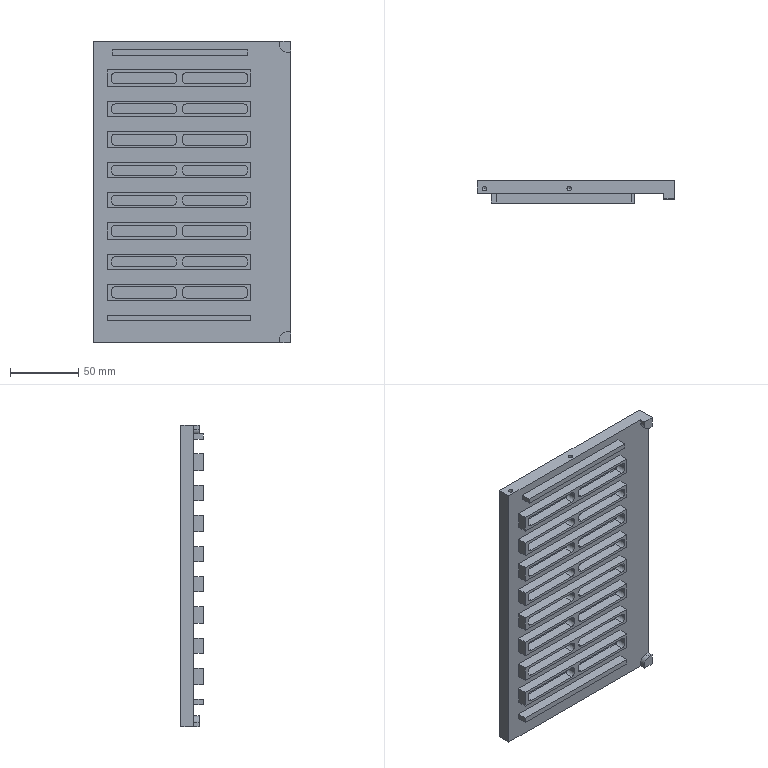NC program | NX | posted with a generic post | part box 144.5 x 16.5 x 221 mm
Lines 4750 to 5825 of 11164:
(CAVITY_MILL_COPY , TOOL : D5-15-D6-50-3T-ROUGH)
N9486 T03 M6
N9488 G54
N9490 G17 G0 G90 X82. Y-0.207 B0. C0. S4500 M3
N9492 G43 Z20. H3
N9494 Z0.533 B-180. C-180.
N9496 G94 G1 Y4.25 Z0.378 F1200.
N9498 Y4.387 Z0.373
N9500 X82.163 Y4.55 Z0.365
N9502 X82.3 Z0.36
N9504 X84.514 Z0.283
N9506 X84.583 Y4.546 Z0.28
N9508 X84.644 Y4.513 Z0.278
N9510 X84.763 Y4.394 Z0.272
N9512 X84.8 Y4.327 Z0.269
N9514 Y-10.463 Z-0.247
N9516 Y-16.75 Z-0.467
N9518 Y-37.75
N9520 X84.79 Y-37.826
N9522 G2 X84.465 Y-38.05 R0.302
N9524 G1 X82.335
N9526 G2 X82.105 Y-37.978 R0.409
N9528 X82. Y-37.75 R0.3
N9530 G1 Y4.25
N9532 G2 X82.3 Y4.55 R0.3
N9534 G1 X84.514
N9536 X84.589 Y4.568
N9538 X84.644 Y4.513
N9540 X84.763 Y4.394
N9542 X84.82 Y4.332
N9544 X84.8 Y4.25
N9546 Y-16.75
N9548 Z0.533
N9550 G0 Z20.
N9552 X82. Y-0.206
N9554 Z0.067
N9556 G1 Y4.387 Z-0.094
N9558 X82.163 Y4.55 Z-0.102
N9560 X84.577 Z-0.186
N9562 X84.644 Y4.513 Z-0.189
N9564 X84.763 Y4.394 Z-0.195
N9566 X84.8 Y4.327 Z-0.197
N9568 Y-16.75 Z-0.933
N9570 Y-37.75
N9572 X84.79 Y-37.825
N9574 G2 X84.5 Y-38.05 R0.3
N9576 G1 X82.335
N9578 G2 X82.105 Y-37.978 R0.409
N9580 X82. Y-37.75 R0.3
N9582 G1 Y4.25
N9584 G2 X82.3 Y4.55 R0.3
N9586 G1 X84.5
N9588 X84.582 Y4.57
N9590 X84.644 Y4.513
N9592 X84.763 Y4.394
N9594 X84.82 Y4.332
N9596 X84.8 Y4.25
N9598 Y-16.75
N9600 Z0.067
N9602 G0 Z20.
N9604 X82. Y-0.206
N9606 Z-0.4
N9608 G1 Y4.25 Z-0.556
N9610 Y4.387 Z-0.56
N9612 X82.163 Y4.55 Z-0.568
N9614 X82.3 Z-0.573
N9616 X84.577 Z-0.653
N9618 X84.644 Y4.513 Z-0.655
N9620 X84.763 Y4.394 Z-0.661
N9622 X84.8 Y4.327 Z-0.664
N9624 Y-16.75 Z-1.4
N9626 Y-37.75
N9628 X84.79 Y-37.825
N9630 G2 X84.5 Y-38.05 R0.3
N9632 G1 X82.335
N9634 G2 X82.105 Y-37.978 R0.409
N9636 X82. Y-37.75 R0.3
N9638 G1 Y4.25
N9640 G2 X82.3 Y4.55 R0.3
N9642 G1 X84.5
N9644 X84.582 Y4.57
N9646 X84.644 Y4.513
N9648 X84.763 Y4.394
N9650 X84.82 Y4.332
N9652 X84.8 Y4.25
N9654 Y-16.75
N9656 Z-0.4
N9658 G0 Z20.
N9660 X82. Y-0.206
N9662 Z-0.867
N9664 G1 Y4.25 Z-1.022
N9666 Y4.387 Z-1.027
N9668 X82.163 Y4.55 Z-1.035
N9670 X82.3 Z-1.04
N9672 X84.577 Z-1.119
N9674 X84.644 Y4.513 Z-1.122
N9676 X84.763 Y4.394 Z-1.128
N9678 X84.8 Y4.327 Z-1.131
N9680 Y-16.75 Z-1.867
N9682 Y-37.75
N9684 X84.79 Y-37.825
N9686 G2 X84.5 Y-38.05 R0.3
N9688 G1 X82.335
N9690 G2 X82.105 Y-37.978 R0.409
N9692 X82. Y-37.75 R0.3
N9694 G1 Y4.25
N9696 G2 X82.3 Y4.55 R0.3
N9698 G1 X84.5
N9700 X84.582 Y4.57
N9702 X84.644 Y4.513
N9704 X84.763 Y4.394
N9706 X84.82 Y4.332
N9708 X84.8 Y4.25
N9710 Y-16.75
N9712 Z-0.867
N9714 G0 Z20.
N9716 X82. Y-0.206
N9718 Z-1.333
N9720 G1 Y4.387 Z-1.494
N9722 X82.163 Y4.55 Z-1.502
N9724 X84.577 Z-1.586
N9726 X84.644 Y4.513 Z-1.589
N9728 X84.763 Y4.394 Z-1.595
N9730 X84.8 Y4.327 Z-1.597
N9732 Y-16.75 Z-2.333
N9734 Y-37.75
N9736 X84.79 Y-37.825
N9738 G2 X84.5 Y-38.05 R0.3
N9740 G1 X82.335
N9742 G2 X82.105 Y-37.978 R0.409
N9744 X82. Y-37.75 R0.3
N9746 G1 Y4.25
N9748 G2 X82.3 Y4.55 R0.3
N9750 G1 X84.5
N9752 X84.582 Y4.57
N9754 X84.644 Y4.513
N9756 X84.763 Y4.394
N9758 X84.82 Y4.332
N9760 X84.8 Y4.25
N9762 Y-16.75
N9764 Z-1.333
N9766 G0 Z20.
N9768 X82. Y-0.206
N9770 Z-1.8
N9772 G1 Y4.387 Z-1.96
N9774 X82.163 Y4.55 Z-1.968
N9776 X84.577 Z-2.053
N9778 X84.644 Y4.513 Z-2.055
N9780 X84.763 Y4.394 Z-2.061
N9782 X84.8 Y4.327 Z-2.064
N9784 Y-16.75 Z-2.8
N9786 Y-37.75
N9788 X84.79 Y-37.825
N9790 G2 X84.5 Y-38.05 R0.3
N9792 G1 X82.335
N9794 G2 X82.105 Y-37.978 R0.409
N9796 X82. Y-37.75 R0.3
N9798 G1 Y4.25
N9800 G2 X82.3 Y4.55 R0.3
N9802 G1 X84.5
N9804 X84.582 Y4.57
N9806 X84.644 Y4.513
N9808 X84.763 Y4.394
N9810 X84.82 Y4.332
N9812 X84.8 Y4.25
N9814 Y-16.75
N9816 Z-1.8
N9818 G0 Z20.
N9820 X82. Y-0.206
N9822 Z-2.3
N9824 G1 Y4.25 Z-2.456
N9826 Y4.387 Z-2.46
N9828 X82.163 Y4.55 Z-2.468
N9830 X82.3 Z-2.473
N9832 X84.577 Z-2.553
N9834 X84.644 Y4.513 Z-2.555
N9836 X84.763 Y4.394 Z-2.561
N9838 X84.8 Y4.327 Z-2.564
N9840 Y-16.75 Z-3.3
N9842 Y-37.75
N9844 X84.79 Y-37.825
N9846 G2 X84.5 Y-38.05 R0.3
N9848 G1 X82.335
N9850 G2 X82.105 Y-37.978 R0.409
N9852 G1 X82.06 Y-37.93
N9854 X81.987 Y-37.855
N9856 X82. Y-37.75
N9858 Y4.25
N9860 G2 X82.3 Y4.55 R0.3
N9862 G1 X84.5
N9864 X84.582 Y4.57
N9866 X84.644 Y4.513
N9868 X84.763 Y4.394
N9870 X84.82 Y4.332
N9872 X84.8 Y4.25
N9874 Y-16.75
N9876 Z-2.3
N9878 G0 Z20.
N9880 X82. Y-0.206
N9882 Z-2.8
N9884 G1 Y4.387 Z-2.96
N9886 X82.163 Y4.55 Z-2.968
N9888 X84.577 Z-3.053
N9890 X84.644 Y4.513 Z-3.055
N9892 X84.763 Y4.394 Z-3.061
N9894 X84.8 Y4.327 Z-3.064
N9896 Y-16.75 Z-3.8
N9898 Y-37.75
N9900 X84.79 Y-37.825
N9902 G2 X84.5 Y-38.05 R0.3
N9904 G1 X82.335
N9906 G2 X82.105 Y-37.978 R0.409
N9908 X82. Y-37.75 R0.3
N9910 G1 Y4.25
N9912 G2 X82.3 Y4.55 R0.3
N9914 G1 X84.5
N9916 X84.582 Y4.57
N9918 X84.644 Y4.513
N9920 X84.763 Y4.394
N9922 X84.82 Y4.332
N9924 X84.8 Y4.25
N9926 Y-16.75
N9928 Z-2.8
N9930 G0 Z20.
N9932 X82. Y-0.206
N9934 Z-3.3
N9936 G1 Y4.387 Z-3.46
N9938 X82.163 Y4.55 Z-3.468
N9940 X84.577 Z-3.553
N9942 X84.644 Y4.513 Z-3.555
N9944 X84.763 Y4.394 Z-3.561
N9946 X84.8 Y4.327 Z-3.564
N9948 Y-16.75 Z-4.3
N9950 Y-37.75
N9952 X84.79 Y-37.825
N9954 G2 X84.5 Y-38.05 R0.3
N9956 G1 X82.335
N9958 G2 X82.105 Y-37.978 R0.409
N9960 X82. Y-37.75 R0.3
N9962 G1 Y4.25
N9964 G2 X82.3 Y4.55 R0.3
N9966 G1 X84.5
N9968 X84.582 Y4.57
N9970 X84.644 Y4.513
N9972 X84.763 Y4.394
N9974 X84.82 Y4.332
N9976 X84.8 Y4.25
N9978 Y-16.75
N9980 Z-3.3
N9982 G0 Z20.
N9984 X82. Y-0.206
N9986 Z-3.8
N9988 G1 Y4.387 Z-3.96
N9990 X82.163 Y4.55 Z-3.968
N9992 X84.577 Z-4.053
N9994 X84.644 Y4.513 Z-4.055
N9996 X84.763 Y4.394 Z-4.061
N9998 X84.8 Y4.327 Z-4.064
N10000 Y-16.75 Z-4.8
N10002 Y-37.75
N10004 X84.79 Y-37.825
N10006 G2 X84.5 Y-38.05 R0.3
N10008 G1 X82.335
N10010 G2 X82.105 Y-37.978 R0.409
N10012 X82. Y-37.75 R0.3
N10014 G1 Y4.25
N10016 G2 X82.3 Y4.55 R0.3
N10018 G1 X84.5
N10020 X84.582 Y4.57
N10022 X84.644 Y4.513
N10024 X84.763 Y4.394
N10026 X84.82 Y4.332
N10028 X84.8 Y4.25
N10030 Y-16.75
N10032 Z-3.8
N10034 G0 Z20.
N10036 X82. Y-0.206
N10038 Z-4.3
N10040 G1 Y4.387 Z-4.46
N10042 X82.163 Y4.55 Z-4.468
N10044 X84.577 Z-4.553
N10046 X84.644 Y4.513 Z-4.555
N10048 X84.763 Y4.394 Z-4.561
N10050 X84.8 Y4.327 Z-4.564
N10052 Y-16.75 Z-5.3
N10054 Y-37.75
N10056 X84.79 Y-37.825
N10058 G2 X84.5 Y-38.05 R0.3
N10060 G1 X82.335
N10062 G2 X82.105 Y-37.978 R0.409
N10064 X82. Y-37.75 R0.3
N10066 G1 Y4.25
N10068 G2 X82.3 Y4.55 R0.3
N10070 G1 X84.5
N10072 X84.582 Y4.57
N10074 X84.644 Y4.513
N10076 X84.763 Y4.394
N10078 X84.82 Y4.332
N10080 X84.8 Y4.25
N10082 Y-16.75
N10084 Z-4.3
N10086 G0 Z20.
N10088 X82. Y-0.206
N10090 Z-4.8
N10092 G1 Y4.387 Z-4.96
N10094 X82.163 Y4.55 Z-4.968
N10096 X84.577 Z-5.053
N10098 X84.644 Y4.513 Z-5.055
N10100 X84.763 Y4.394 Z-5.061
N10102 X84.8 Y4.327 Z-5.064
N10104 Y-16.75 Z-5.8
N10106 Y-37.75
N10108 X84.79 Y-37.825
N10110 G2 X84.5 Y-38.05 R0.3
N10112 G1 X82.334
N10114 G2 X82.105 Y-37.978 R0.409
N10116 X82. Y-37.75 R0.3
N10118 G1 Y4.25
N10120 G2 X82.3 Y4.55 R0.3
N10122 G1 X84.5
N10124 X84.582 Y4.57
N10126 X84.644 Y4.513
N10128 X84.763 Y4.394
N10130 X84.82 Y4.332
N10132 X84.8 Y4.25
N10134 Y-16.75
N10136 Z-4.8
N10138 G0 Z20.
N10140 X82. Y-0.206
N10142 Z-5.3
N10144 G1 Y4.387 Z-5.46
N10146 X82.163 Y4.55 Z-5.468
N10148 X84.577 Z-5.553
N10150 X84.644 Y4.513 Z-5.555
N10152 X84.763 Y4.394 Z-5.561
N10154 X84.8 Y4.327 Z-5.564
N10156 Y-16.75 Z-6.3
N10158 Y-37.75
N10160 X84.79 Y-37.825
N10162 G2 X84.5 Y-38.05 R0.3
N10164 G1 X82.334
N10166 G2 X82.105 Y-37.978 R0.409
N10168 X82. Y-37.75 R0.3
N10170 G1 Y4.25
N10172 G2 X82.3 Y4.55 R0.3
N10174 G1 X84.5
N10176 X84.582 Y4.57
N10178 X84.644 Y4.513
N10180 X84.763 Y4.394
N10182 X84.82 Y4.332
N10184 X84.8 Y4.25
N10186 Y-16.75
N10188 Z-5.3
N10190 G0 Z20.
N10192 X82. Y-0.206
N10194 Z-5.8
N10196 G1 Y4.387 Z-5.96
N10198 X82.163 Y4.55 Z-5.968
N10200 X84.577 Z-6.053
N10202 X84.644 Y4.513 Z-6.055
N10204 X84.763 Y4.394 Z-6.061
N10206 X84.8 Y4.327 Z-6.064
N10208 Y-16.75 Z-6.8
N10210 Y-37.75
N10212 X84.79 Y-37.825
N10214 G2 X84.5 Y-38.05 R0.3
N10216 G1 X82.334
N10218 G2 X82.105 Y-37.978 R0.409
N10220 X82. Y-37.75 R0.3
N10222 G1 Y4.25
N10224 G2 X82.3 Y4.55 R0.3
N10226 G1 X84.5
N10228 X84.582 Y4.57
N10230 X84.644 Y4.513
N10232 X84.763 Y4.394
N10234 X84.82 Y4.332
N10236 X84.8 Y4.25
N10238 Y-16.75
N10240 Z-5.8
N10242 G0 Z20.
N10244 X61.8 Y-32.367
N10246 Z0.533
N10248 G1 Y-37.75 Z0.345
N10250 Y-37.887 Z0.341
N10252 X61.638 Y-38.05 Z0.333
N10254 X61.501 Z0.328
N10256 X61.261 Z0.319
N10258 X60.259 Y-38.047 Z0.284
N10260 X60.12 Y-38.023 Z0.279
N10262 X60.027 Y-37.93 Z0.275
N10264 X60. Y-37.771 Z0.269
N10266 Y-16.697 Z-0.467
N10268 Y4.25
N10270 X60.036 Y4.392
N10272 G2 X60.3 Y4.55 R0.3
N10274 G1 X61.5
N10276 G2 X61.8 Y4.25 R0.3
N10278 G1 Y-37.75
N10280 G2 X61.501 Y-38.05 R0.3
N10282 G1 X61.261
N10284 X60.259 Y-38.047
N10286 G2 X60. Y-37.75 R0.316
N10288 G1 Y-16.697
N10290 Z0.533
N10292 G0 Z20.
N10294 X61.8 Y-32.367
N10296 Z0.067
N10298 G1 Y-37.75 Z-0.121
N10300 Y-37.887 Z-0.126
N10302 X61.638 Y-38.05 Z-0.134
N10304 X61.501 Z-0.139
N10306 X61.301 Z-0.146
N10308 X60.259 Y-38.047 Z-0.182
N10310 X60.12 Y-38.023 Z-0.187
N10312 X60.027 Y-37.93 Z-0.192
N10314 X60. Y-37.771 Z-0.197
N10316 Y-16.697 Z-0.933
N10318 Y4.25
N10320 X60.036 Y4.392
N10322 G2 X60.3 Y4.55 R0.3
N10324 G1 X61.5
N10326 G2 X61.8 Y4.25 R0.3
N10328 G1 Y-37.75
N10330 G2 X61.501 Y-38.05 R0.3
N10332 G1 X61.301
N10334 X60.259 Y-38.047
N10336 G2 X60. Y-37.75 R0.316
N10338 G1 Y-16.697
N10340 Z0.067
N10342 G0 Z20.
N10344 X61.8 Y-32.367
N10346 Z-0.4
N10348 G1 Y-37.75 Z-0.588
N10350 Y-37.887 Z-0.593
N10352 X61.638 Y-38.05 Z-0.601
N10354 X61.5 Z-0.606
N10356 X61.341 Z-0.611
N10358 X60.259 Y-38.047 Z-0.649
N10360 X60.12 Y-38.023 Z-0.654
N10362 X60.027 Y-37.93 Z-0.658
N10364 X60. Y-37.771 Z-0.664
N10366 Y-16.697 Z-1.4
N10368 Y4.25
N10370 X60.036 Y4.392
N10372 G2 X60.3 Y4.55 R0.3
N10374 G1 X61.5
N10376 G2 X61.8 Y4.25 R0.3
N10378 G1 Y-37.75
N10380 G2 X61.5 Y-38.05 R0.3
N10382 G1 X61.341
N10384 X60.259 Y-38.047
N10386 G2 X60. Y-37.75 R0.316
N10388 G1 Y-16.697
N10390 Z-0.4
N10392 G0 Z20.
N10394 X61.8 Y-32.367
N10396 Z-0.867
N10398 G1 Y-37.75 Z-1.055
N10400 Y-37.887 Z-1.059
N10402 X61.638 Y-38.05 Z-1.067
N10404 X61.5 Z-1.072
N10406 X61.381 Z-1.076
N10408 X60.259 Y-38.047 Z-1.116
N10410 X60.12 Y-38.023 Z-1.121
N10412 X60.027 Y-37.93 Z-1.125
N10414 X60. Y-37.771 Z-1.131
N10416 Y-16.697 Z-1.867
N10418 Y4.25
N10420 X60.036 Y4.392
N10422 G2 X60.3 Y4.55 R0.3
N10424 G1 X61.5
N10426 G2 X61.8 Y4.25 R0.3
N10428 G1 Y-37.75
N10430 G2 X61.5 Y-38.05 R0.3
N10432 G1 X61.381
N10434 X60.259 Y-38.047
N10436 G2 X60. Y-37.75 R0.316
N10438 G1 Y-16.697
N10440 Z-0.867
N10442 G0 Z20.
N10444 X61.8 Y-32.367
N10446 Z-1.333
N10448 G1 Y-37.75 Z-1.521
N10450 Y-37.887 Z-1.526
N10452 X61.638 Y-38.05 Z-1.534
N10454 X61.5 Z-1.539
N10456 X61.421 Z-1.542
N10458 X60.259 Y-38.047 Z-1.582
N10460 X60.12 Y-38.023 Z-1.587
N10462 X60.027 Y-37.93 Z-1.592
N10464 X60. Y-37.771 Z-1.597
N10466 Y-16.697 Z-2.333
N10468 Y4.25
N10470 X60.036 Y4.392
N10472 G2 X60.3 Y4.55 R0.3
N10474 G1 X61.5
N10476 G2 X61.8 Y4.25 R0.3
N10478 G1 Y-37.75
N10480 G2 X61.5 Y-38.05 R0.3
N10482 G1 X61.421
N10484 X60.259 Y-38.047
N10486 G2 X60. Y-37.75 R0.316
N10488 G1 Y-16.697
N10490 Z-1.333
N10492 G0 Z20.
N10494 X61.8 Y-32.367
N10496 Z-1.8
N10498 G1 Y-37.75 Z-1.988
N10500 Y-37.887 Z-1.993
N10502 X61.638 Y-38.05 Z-2.001
N10504 X61.46 Z-2.007
N10506 X60.259 Y-38.047 Z-2.049
N10508 X60.12 Y-38.023 Z-2.054
N10510 X60.027 Y-37.93 Z-2.058
N10512 X60. Y-37.771 Z-2.064
N10514 Y-16.697 Z-2.8
N10516 Y4.25
N10518 X60.036 Y4.392
N10520 G2 X60.3 Y4.55 R0.3
N10522 G1 X61.5
N10524 G2 X61.8 Y4.25 R0.3
N10526 G1 Y-37.75
N10528 G2 X61.46 Y-38.05 R0.303
N10530 G1 X60.259 Y-38.047
N10532 G2 X60. Y-37.75 R0.316
N10534 G1 Y-16.697
N10536 Z-1.8
N10538 G0 Z20.
N10540 X61.8 Y-32.366
N10542 Z-2.3
N10544 G1 Y-37.75 Z-2.488
N10546 Y-37.887 Z-2.493
N10548 X61.657 Y-38.04 Z-2.5
N10550 X61.46 Y-38.05 Z-2.507
N10552 X60.259 Y-38.047 Z-2.549
N10554 X60.12 Y-38.023 Z-2.554
N10556 X60.027 Y-37.93 Z-2.558
N10558 X60. Y-37.771 Z-2.564
N10560 Y-16.697 Z-3.3
N10562 Y4.25
N10564 X60.036 Y4.392
N10566 G2 X60.3 Y4.55 R0.3
N10568 G1 X61.5
N10570 G2 X61.8 Y4.25 R0.3
N10572 G1 Y-37.75
N10574 G2 X61.46 Y-38.05 R0.303
N10576 G1 X60.259 Y-38.047
N10578 G2 X60. Y-37.75 R0.316
N10580 G1 Y-16.697
N10582 Z-2.3
N10584 G0 Z20.
N10586 X61.8 Y-32.367
N10588 Z-2.8
N10590 G1 Y-37.75 Z-2.988
N10592 Y-37.887 Z-2.993
N10594 X61.637 Y-38.05 Z-3.001
N10596 X61.5 Z-3.006
N10598 X60.259 Y-38.047 Z-3.049
N10600 X60.12 Y-38.023 Z-3.054
N10602 X60.027 Y-37.93 Z-3.058
N10604 X60. Y-37.771 Z-3.064
N10606 Y-16.697 Z-3.8
N10608 Y4.25
N10610 X60.036 Y4.392
N10612 G2 X60.3 Y4.55 R0.3
N10614 G1 X61.5
N10616 G2 X61.8 Y4.25 R0.3
N10618 G1 Y-37.75
N10620 G2 X61.5 Y-38.05 R0.3
N10622 G1 X60.259 Y-38.047
N10624 G2 X60. Y-37.75 R0.316
N10626 G1 Y-16.697
N10628 Z-2.8
N10630 G0 Z20.
N10632 X61.8 Y-32.367
N10634 Z-3.3
N10636 G1 Y-37.75 Z-3.488
N10638 Y-37.887 Z-3.493
N10640 X61.637 Y-38.05 Z-3.501
N10642 X61.5 Z-3.506
N10644 X60.259 Y-38.047 Z-3.549
N10646 X60.12 Y-38.023 Z-3.554
N10648 X60.027 Y-37.93 Z-3.558
N10650 X60. Y-37.771 Z-3.564
N10652 Y-16.697 Z-4.3
N10654 Y4.25
N10656 X60.036 Y4.392
N10658 G2 X60.3 Y4.55 R0.3
N10660 G1 X61.5
N10662 G2 X61.8 Y4.25 R0.3
N10664 G1 Y-37.75
N10666 G2 X61.5 Y-38.05 R0.3
N10668 G1 X60.259 Y-38.047
N10670 G2 X60. Y-37.75 R0.316
N10672 G1 Y-16.697
N10674 Z-3.3
N10676 G0 Z20.
N10678 X61.8 Y-32.367
N10680 Z-3.8
N10682 G1 Y-37.75 Z-3.988
N10684 Y-37.887 Z-3.993
N10686 X61.637 Y-38.05 Z-4.001
N10688 X61.5 Z-4.006
N10690 X60.259 Y-38.047 Z-4.049
N10692 X60.12 Y-38.023 Z-4.054
N10694 X60.027 Y-37.93 Z-4.058
N10696 X60. Y-37.771 Z-4.064
N10698 Y-16.697 Z-4.8
N10700 Y4.25
N10702 X60.036 Y4.392
N10704 G2 X60.3 Y4.55 R0.3
N10706 G1 X61.5
N10708 G2 X61.8 Y4.25 R0.3
N10710 G1 Y-37.75
N10712 G2 X61.5 Y-38.05 R0.3
N10714 G1 X60.259 Y-38.047
N10716 G2 X60. Y-37.75 R0.316
N10718 G1 Y-16.697
N10720 Z-3.8
N10722 G0 Z20.
N10724 X61.8 Y-32.367
N10726 Z-4.3
N10728 G1 Y-37.75 Z-4.488
N10730 Y-37.887 Z-4.493
N10732 X61.637 Y-38.05 Z-4.501
N10734 X61.5 Z-4.506
N10736 X60.259 Y-38.047 Z-4.549
N10738 X60.12 Y-38.023 Z-4.554
N10740 X60.027 Y-37.93 Z-4.558
N10742 X60. Y-37.771 Z-4.564
N10744 Y-16.697 Z-5.3
N10746 Y4.25
N10748 X60.036 Y4.392
N10750 G2 X60.3 Y4.55 R0.3
N10752 G1 X61.5
N10754 G2 X61.8 Y4.25 R0.3
N10756 G1 Y-37.75
N10758 G2 X61.5 Y-38.05 R0.3
N10760 G1 X60.259 Y-38.047
N10762 G2 X60. Y-37.75 R0.316
N10764 G1 Y-16.697
N10766 Z-4.3
N10768 G0 Z20.
N10770 X61.8 Y-32.367
N10772 Z-4.8
N10774 G1 Y-37.75 Z-4.988
N10776 Y-37.887 Z-4.993
N10778 X61.637 Y-38.05 Z-5.001
N10780 X61.5 Z-5.006
N10782 X60.259 Y-38.047 Z-5.049
N10784 X60.12 Y-38.023 Z-5.054
N10786 X60.027 Y-37.93 Z-5.058
N10788 X60. Y-37.771 Z-5.064
N10790 Y-16.697 Z-5.8
N10792 Y4.25
N10794 X60.036 Y4.392
N10796 G2 X60.3 Y4.55 R0.3
N10798 G1 X61.5
N10800 G2 X61.8 Y4.25 R0.3
N10802 G1 Y-37.75
N10804 G2 X61.5 Y-38.05 R0.3
N10806 G1 X60.259 Y-38.047
N10808 G2 X60. Y-37.75 R0.316
N10810 G1 Y-16.697
N10812 Z-4.8
N10814 G0 Z20.
N10816 X61.8 Y-32.367
N10818 Z-5.3
N10820 G1 Y-37.75 Z-5.488
N10822 Y-37.887 Z-5.493
N10824 X61.637 Y-38.05 Z-5.501
N10826 X61.5 Z-5.506
N10828 X60.259 Y-38.047 Z-5.549
N10830 X60.12 Y-38.023 Z-5.554
N10832 X60.027 Y-37.93 Z-5.558
N10834 X60. Y-37.771 Z-5.564
N10836 Y-16.697 Z-6.3
N10838 Y4.25
N10840 X60.036 Y4.392
N10842 G2 X60.3 Y4.55 R0.3
N10844 G1 X61.5
N10846 G2 X61.8 Y4.25 R0.3
N10848 G1 Y-37.75
N10850 G2 X61.5 Y-38.05 R0.3
N10852 G1 X60.259 Y-38.047
N10854 G2 X60. Y-37.75 R0.316
N10856 G1 Y-16.697
N10858 Z-5.3
N10860 G0 Z20.
N10862 X61.8 Y-32.367
N10864 Z-5.8
N10866 G1 Y-37.75 Z-5.988
N10868 Y-37.887 Z-5.993
N10870 X61.637 Y-38.05 Z-6.001
N10872 X61.5 Z-6.006
N10874 X60.259 Y-38.047 Z-6.049
N10876 X60.12 Y-38.023 Z-6.054
N10878 X60.027 Y-37.93 Z-6.058
N10880 X60. Y-37.771 Z-6.064
N10882 Y-16.697 Z-6.8
N10884 Y4.25
N10886 X60.036 Y4.392
N10888 G2 X60.3 Y4.55 R0.3
N10890 G1 X61.5
N10892 G2 X61.8 Y4.25 R0.3
N10894 G1 Y-37.75
N10896 G2 X61.5 Y-38.05 R0.3
N10898 G1 X60.259 Y-38.047
N10900 G2 X60. Y-37.75 R0.316
N10902 G1 Y-16.697
N10904 Z-5.8
N10906 G0 Z20.
N10908 X37. Y-0.18
N10910 Z0.533
N10912 G1 X37.002 Y4.289 Z0.377
N10914 X37.035 Y4.446 Z0.372
N10916 X37.163 Y4.55 Z0.366
N10918 X37.3 Z0.361
N10920 X39.637 Z0.279
N10922 X39.8 Y4.387 Z0.271
N10924 Y-16.75 Z-0.467
N10926 Y-37.75
N10928 G2 X39.5 Y-38.05 R0.3
N10930 G1 X37.263 Y-38.048
N10932 X37.214 Y-38.037
N10934 G2 X37. Y-37.75 R0.3
N10936 G1 Y4.266
N10938 X37.006 Y4.312
N10940 G2 X37.3 Y4.55 R0.3
N10942 G1 X39.5
N10944 G2 X39.8 Y4.25 R0.3
N10946 G1 Y-16.75
N10948 Z0.533
N10950 G0 Z20.
N10952 X37. Y-0.177
N10954 Z0.067
N10956 G1 Y4.266 Z-0.089
N10958 X37.008 Y4.403 Z-0.093
N10960 X37.163 Y4.55 Z-0.101
N10962 X39.637 Z-0.187
N10964 X39.8 Y4.387 Z-0.195
N10966 Y-16.75 Z-0.933
N10968 Y-37.75
N10970 G2 X39.5 Y-38.05 R0.3
N10972 G1 X37.271 Y-38.049
N10974 G2 X37. Y-37.75 R0.3
N10976 G1 Y4.266
N10978 G2 X37.3 Y4.55 R0.3
N10980 G1 X39.5
N10982 G2 X39.8 Y4.25 R0.3
N10984 G1 Y-16.75
N10986 Z0.067
N10988 G0 Z20.
N10990 X37. Y-0.177
N10992 Z-0.4
N10994 G1 Y4.266 Z-0.555
N10996 X37.008 Y4.403 Z-0.56
N10998 X37.163 Y4.55 Z-0.567
N11000 X39.637 Z-0.654
N11002 X39.8 Y4.387 Z-0.662
N11004 Y-16.75 Z-1.4
N11006 Y-37.75
N11008 G2 X39.5 Y-38.05 R0.3
N11010 G1 X37.271 Y-38.049
N11012 G2 X37. Y-37.75 R0.3
N11014 G1 Y4.266
N11016 G2 X37.3 Y4.55 R0.3
N11018 G1 X39.5
N11020 G2 X39.8 Y4.25 R0.3
N11022 G1 Y-16.75
N11024 Z-0.4
N11026 G0 Z20.
N11028 X37. Y-0.177
N11030 Z-0.867
N11032 G1 Y4.266 Z-1.022
N11034 X37.008 Y4.403 Z-1.027
N11036 X37.163 Y4.55 Z-1.034
N11038 X39.637 Z-1.121
N11040 X39.8 Y4.387 Z-1.129
N11042 Y-16.75 Z-1.867
N11044 Y-37.75
N11046 G2 X39.5 Y-38.05 R0.3
N11048 G1 X37.271 Y-38.049
N11050 G2 X37. Y-37.75 R0.3
N11052 G1 Y4.266
N11054 G2 X37.3 Y4.55 R0.3
N11056 G1 X39.5
N11058 G2 X39.8 Y4.25 R0.3
N11060 G1 Y-16.75
N11062 Z-0.867
N11064 G0 Z20.
N11066 X37. Y-0.177
N11068 Z-1.333
N11070 G1 Y4.266 Z-1.489
N11072 X37.008 Y4.403 Z-1.493
N11074 X37.163 Y4.55 Z-1.501
N11076 X39.637 Z-1.587
N11078 X39.8 Y4.387 Z-1.595
N11080 Y-16.75 Z-2.333
N11082 Y-37.75
N11084 G2 X39.5 Y-38.05 R0.3
N11086 G1 X37.271 Y-38.049
N11088 G2 X37. Y-37.75 R0.3
N11090 G1 Y4.266
N11092 G2 X37.3 Y4.55 R0.3
N11094 G1 X39.5
N11096 G2 X39.8 Y4.25 R0.3
N11098 G1 Y-16.75
N11100 Z-1.333
N11102 G0 Z20.
N11104 X37. Y-0.177
N11106 Z-1.8
N11108 G1 Y4.266 Z-1.955
N11110 X37.008 Y4.403 Z-1.96
N11112 X37.163 Y4.55 Z-1.967
N11114 X39.637 Z-2.054
N11116 X39.8 Y4.387 Z-2.062
N11118 Y-16.75 Z-2.8
N11120 Y-37.75
N11122 G2 X39.5 Y-38.05 R0.3
N11124 G1 X37.271 Y-38.049
N11126 G2 X37. Y-37.75 R0.3
N11128 G1 Y4.266
N11130 G2 X37.3 Y4.55 R0.3
N11132 G1 X39.5
N11134 G2 X39.8 Y4.25 R0.3
N11136 G1 Y-16.75
N11138 Z-1.8
N11140 G0 Z20.
N11142 X37. Y-0.177
N11144 Z-2.3
N11146 G1 Y4.266 Z-2.455
N11148 X37.008 Y4.403 Z-2.46
N11150 X37.163 Y4.55 Z-2.467
N11152 X39.637 Z-2.554
N11154 X39.8 Y4.387 Z-2.562
N11156 Y-16.75 Z-3.3
N11158 Y-37.75
N11160 G2 X39.5 Y-38.05 R0.3
N11162 G1 X37.271 Y-38.049
N11164 G2 X37. Y-37.75 R0.3
N11166 G1 Y4.266
N11168 G2 X37.3 Y4.55 R0.3
N11170 G1 X39.5
N11172 G2 X39.8 Y4.25 R0.3
N11174 G1 Y-16.75
N11176 Z-2.3
N11178 G0 Z20.
N11180 X37. Y-0.177
N11182 Z-2.8
N11184 G1 Y4.266 Z-2.955
N11186 X37.008 Y4.403 Z-2.96
N11188 X37.163 Y4.55 Z-2.967
N11190 X39.637 Z-3.054
N11192 X39.8 Y4.387 Z-3.062
N11194 Y-16.75 Z-3.8
N11196 Y-37.75
N11198 G2 X39.5 Y-38.05 R0.3
N11200 G1 X37.271 Y-38.049
N11202 G2 X37. Y-37.75 R0.3
N11204 G1 Y4.266
N11206 G2 X37.3 Y4.55 R0.3
N11208 G1 X39.5
N11210 G2 X39.8 Y4.25 R0.3
N11212 G1 Y-16.75
N11214 Z-2.8
N11216 G0 Z20.
N11218 X37. Y-0.177
N11220 Z-3.3
N11222 G1 Y4.266 Z-3.455
N11224 X37.008 Y4.403 Z-3.46
N11226 X37.163 Y4.55 Z-3.467
N11228 X39.637 Z-3.554
N11230 X39.8 Y4.387 Z-3.562
N11232 Y-16.75 Z-4.3
N11234 Y-37.75
N11236 G2 X39.5 Y-38.05 R0.3
N11238 G1 X37.271 Y-38.049
N11240 G2 X37. Y-37.75 R0.3
N11242 G1 Y4.266
N11244 G2 X37.3 Y4.55 R0.3
N11246 G1 X39.5
N11248 G2 X39.8 Y4.25 R0.3
N11250 G1 Y-16.75
N11252 Z-3.3
N11254 G0 Z20.
N11256 X37. Y-0.177
N11258 Z-3.8
N11260 G1 Y4.266 Z-3.955
N11262 X37.008 Y4.403 Z-3.96
N11264 X37.163 Y4.55 Z-3.967
N11266 X39.637 Z-4.054
N11268 X39.8 Y4.387 Z-4.062
N11270 Y-16.75 Z-4.8
N11272 Y-37.75
N11274 G2 X39.5 Y-38.05 R0.3
N11276 G1 X37.271 Y-38.049
N11278 G2 X37. Y-37.75 R0.3
N11280 G1 Y4.266
N11282 G2 X37.3 Y4.55 R0.3
N11284 G1 X39.5
N11286 G2 X39.8 Y4.25 R0.3
N11288 G1 Y-16.75
N11290 Z-3.8
N11292 G0 Z20.
N11294 X37. Y-0.177
N11296 Z-4.3
N11298 G1 Y4.266 Z-4.455
N11300 X37.008 Y4.403 Z-4.46
N11302 X37.163 Y4.55 Z-4.467
N11304 X39.637 Z-4.554
N11306 X39.8 Y4.387 Z-4.562
N11308 Y-16.75 Z-5.3
N11310 Y-37.75
N11312 G2 X39.5 Y-38.05 R0.3
N11314 G1 X37.271 Y-38.049
N11316 G2 X37. Y-37.75 R0.3
N11318 G1 Y4.266
N11320 G2 X37.3 Y4.55 R0.3
N11322 G1 X39.5
N11324 G2 X39.8 Y4.25 R0.3
N11326 G1 Y-16.75
N11328 Z-4.3
N11330 G0 Z20.
N11332 X37. Y-0.177
N11334 Z-4.8
N11336 G1 Y4.266 Z-4.955
N11338 X37.008 Y4.403 Z-4.96
N11340 X37.163 Y4.55 Z-4.967
N11342 X39.637 Z-5.054
N11344 X39.8 Y4.387 Z-5.062
N11346 Y-16.75 Z-5.8
N11348 Y-37.75
N11350 G2 X39.5 Y-38.05 R0.3
N11352 G1 X37.271 Y-38.049
N11354 G2 X37. Y-37.75 R0.3
N11356 G1 Y4.266
N11358 G2 X37.3 Y4.55 R0.3
N11360 G1 X39.5
N11362 G2 X39.8 Y4.25 R0.3
N11364 G1 Y-16.75
N11366 Z-4.8
N11368 G0 Z20.
N11370 X37. Y-0.177
N11372 Z-5.3
N11374 G1 Y4.266 Z-5.455
N11376 X37.008 Y4.403 Z-5.46
N11378 X37.163 Y4.55 Z-5.467
N11380 X39.637 Z-5.554
N11382 X39.8 Y4.387 Z-5.562
N11384 Y-16.75 Z-6.3
N11386 Y-37.75
N11388 G2 X39.5 Y-38.05 R0.3
N11390 G1 X37.271 Y-38.049
N11392 G2 X37. Y-37.75 R0.3
N11394 G1 Y4.266
N11396 G2 X37.3 Y4.55 R0.3
N11398 G1 X39.5
N11400 G2 X39.8 Y4.25 R0.3
N11402 G1 Y-16.75
N11404 Z-5.3
N11406 G0 Z20.
N11408 X37. Y-0.177
N11410 Z-5.8
N11412 G1 Y4.266 Z-5.955
N11414 X37.008 Y4.403 Z-5.96
N11416 X37.163 Y4.55 Z-5.967
N11418 X39.637 Z-6.054
N11420 X39.8 Y4.387 Z-6.062
N11422 Y-16.75 Z-6.8
N11424 Y-37.75
N11426 G2 X39.5 Y-38.05 R0.3
N11428 G1 X37.271 Y-38.049
N11430 G2 X37. Y-37.75 R0.3
N11432 G1 Y4.266
N11434 G2 X37.3 Y4.55 R0.3
N11436 G1 X39.5
N11438 G2 X39.8 Y4.25 R0.3
N11440 G1 Y-16.75
N11442 Z-5.8
N11444 G0 Z20.
N11446 X16.8 Y-32.33
N11448 Z0.533
N11450 G1 Y-37.75 Z0.344
N11452 Y-37.887 Z0.339
N11454 X16.637 Y-38.05 Z0.331
N11456 X16.5 Z0.326
N11458 X15.301 Z0.285
N11460 X15.163 Y-38.049 Z0.28
N11462 X15.001 Y-37.887 Z0.272
N11464 X15. Y-37.749 Z0.267
N11466 Y-16.741 Z-0.467
N11468 Y4.266
N11470 G2 X15.3 Y4.55 R0.3
N11472 G1 X16.5
N11474 G2 X16.8 Y4.25 R0.3
N11476 G1 Y-37.75
N11478 G2 X16.5 Y-38.05 R0.3
N11480 G1 X15.301
N11482 G2 X15. Y-37.749 R0.303
N11484 G1 Y-16.741
N11486 Z0.533
N11488 G0 Z20.
N11490 X16.8 Y-32.33
N11492 Z0.067
N11494 G1 Y-37.75 Z-0.123
N11496 Y-37.887 Z-0.127
N11498 X16.637 Y-38.05 Z-0.135
N11500 X16.5 Z-0.14
N11502 X15.301 Z-0.182
N11504 X15.163 Y-38.049 Z-0.187
N11506 X15.001 Y-37.887 Z-0.195
N11508 X15. Y-37.749 Z-0.2
N11510 Y-16.741 Z-0.933
N11512 Y4.266
N11514 G2 X15.3 Y4.55 R0.3
N11516 G1 X16.5
N11518 G2 X16.8 Y4.25 R0.3
N11520 G1 Y-37.75
N11522 G2 X16.5 Y-38.05 R0.3
N11524 G1 X15.301
N11526 G2 X15. Y-37.749 R0.303
N11528 G1 Y-16.741
N11530 Z0.067
N11532 G0 Z20.
N11534 X16.8 Y-32.33
N11536 Z-0.4
N11538 G1 Y-37.75 Z-0.589
N11540 Y-37.887 Z-0.594
N11542 X16.637 Y-38.05 Z-0.602
N11544 X16.5 Z-0.607
N11546 X15.301 Z-0.649
N11548 X15.163 Y-38.049 Z-0.654
N11550 X15.001 Y-37.887 Z-0.662
N11552 X15. Y-37.749 Z-0.666
N11554 Y-16.741 Z-1.4
N11556 Y4.266
N11558 G2 X15.3 Y4.55 R0.3
N11560 G1 X16.5
N11562 G2 X16.8 Y4.25 R0.3
N11564 G1 Y-37.75
N11566 G2 X16.5 Y-38.05 R0.3
N11568 G1 X15.301
N11570 G2 X15. Y-37.749 R0.303
N11572 G1 Y-16.741
N11574 Z-0.4
N11576 G0 Z20.
N11578 X16.8 Y-32.33
N11580 Z-0.867
N11582 G1 Y-37.75 Z-1.056
N11584 Y-37.887 Z-1.061
N11586 X16.637 Y-38.05 Z-1.069
N11588 X16.5 Z-1.074
N11590 X15.301 Z-1.115
N11592 X15.163 Y-38.049 Z-1.12
N11594 X15.001 Y-37.887 Z-1.128
N11596 X15. Y-37.749 Z-1.133
N11598 Y-16.741 Z-1.867
N11600 Y4.266
N11602 G2 X15.3 Y4.55 R0.3
N11604 G1 X16.5
N11606 G2 X16.8 Y4.25 R0.3
N11608 G1 Y-37.75
N11610 G2 X16.5 Y-38.05 R0.3
N11612 G1 X15.301
N11614 G2 X15. Y-37.749 R0.303
N11616 G1 Y-16.741
N11618 Z-0.867
N11620 G0 Z20.
N11622 X16.8 Y-32.33
N11624 Z-1.333
N11626 G1 Y-37.75 Z-1.523
N11628 Y-37.887 Z-1.527
N11630 X16.637 Y-38.05 Z-1.535